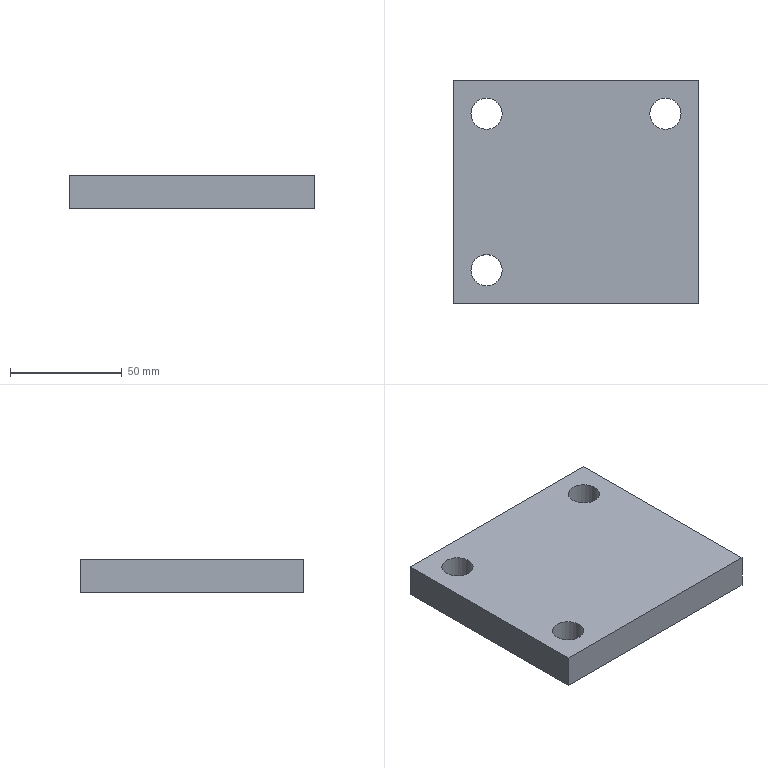Part | NX | features solid 2 | 1 solid | 9 faces | box 110 x 100 x 15 mm | volume 158073 mm3 | plane 6 | cylinder 3 | commonest cylinder face diameters 14 x3
STEP:
#1=CARTESIAN_POINT('',(625.,-751.,-305.));
#2=VERTEX_POINT('',#1);
#3=CARTESIAN_POINT('',(625.,-851.,-305.));
#4=VERTEX_POINT('',#3);
#5=CARTESIAN_POINT('',(625.,-751.,-305.));
#6=DIRECTION('',(0.,1.,0.));
#7=VECTOR('',#6,1000.);
#8=LINE('',#5,#7);
#9=EDGE_CURVE('',#2,#4,#8,.F.);
#10=ORIENTED_EDGE('',*,*,#9,.F.);
#11=CARTESIAN_POINT('',(735.,-751.,-305.));
#12=VERTEX_POINT('',#11);
#13=CARTESIAN_POINT('',(685.,-751.,-305.));
#14=DIRECTION('',(1.,0.,0.));
#15=VECTOR('',#14,1000.);
#16=LINE('',#13,#15);
#17=EDGE_CURVE('',#2,#12,#16,.T.);
#18=ORIENTED_EDGE('',*,*,#17,.T.);
#19=CARTESIAN_POINT('',(735.,-851.,-305.));
#20=VERTEX_POINT('',#19);
#21=CARTESIAN_POINT('',(735.,-842.5,-305.));
#22=DIRECTION('',(0.,-1.,0.));
#23=VECTOR('',#22,1000.);
#24=LINE('',#21,#23);
#25=EDGE_CURVE('',#12,#20,#24,.T.);
#26=ORIENTED_EDGE('',*,*,#25,.T.);
#27=CARTESIAN_POINT('',(685.,-851.,-305.));
#28=DIRECTION('',(1.,0.,0.));
#29=VECTOR('',#28,1000.);
#30=LINE('',#27,#29);
#31=EDGE_CURVE('',#4,#20,#30,.T.);
#32=ORIENTED_EDGE('',*,*,#31,.F.);
#33=EDGE_LOOP('',(#10,#18,#26,#32));
#34=FACE_BOUND('',#33,.T.);
#35=CARTESIAN_POINT('',(633.,-766.,-305.));
#36=VERTEX_POINT('',#35);
#37=CARTESIAN_POINT('',(640.,-766.,-305.));
#38=DIRECTION('',(0.,0.,-1.));
#39=DIRECTION('',(-1.,0.,0.));
#40=AXIS2_PLACEMENT_3D('',#37,#38,#39);
#41=CIRCLE('',#40,7.);
#42=EDGE_CURVE('',#36,#36,#41,.T.);
#43=ORIENTED_EDGE('',*,*,#42,.F.);
#44=EDGE_LOOP('',(#43));
#45=FACE_BOUND('',#44,.T.);
#46=CARTESIAN_POINT('',(713.,-766.,-305.));
#47=VERTEX_POINT('',#46);
#48=CARTESIAN_POINT('',(720.,-766.,-305.));
#49=DIRECTION('',(0.,0.,-1.));
#50=DIRECTION('',(-1.,0.,0.));
#51=AXIS2_PLACEMENT_3D('',#48,#49,#50);
#52=CIRCLE('',#51,7.);
#53=EDGE_CURVE('',#47,#47,#52,.T.);
#54=ORIENTED_EDGE('',*,*,#53,.F.);
#55=EDGE_LOOP('',(#54));
#56=FACE_BOUND('',#55,.T.);
#57=CARTESIAN_POINT('',(633.,-836.,-305.));
#58=VERTEX_POINT('',#57);
#59=CARTESIAN_POINT('',(640.,-836.,-305.));
#60=DIRECTION('',(0.,0.,-1.));
#61=DIRECTION('',(-1.,0.,0.));
#62=AXIS2_PLACEMENT_3D('',#59,#60,#61);
#63=CIRCLE('',#62,7.);
#64=EDGE_CURVE('',#58,#58,#63,.T.);
#65=ORIENTED_EDGE('',*,*,#64,.F.);
#66=EDGE_LOOP('',(#65));
#67=FACE_BOUND('',#66,.T.);
#68=CARTESIAN_POINT('',(685.,-842.5,-305.));
#69=DIRECTION('',(0.,0.,-1.));
#70=DIRECTION('',(1.,0.,0.));
#71=AXIS2_PLACEMENT_3D('',#68,#69,#70);
#72=PLANE('',#71);
#73=ADVANCED_FACE('',(#34,#45,#56,#67),#72,.T.);
#74=CARTESIAN_POINT('',(735.,-751.,-290.));
#75=VERTEX_POINT('',#74);
#76=CARTESIAN_POINT('',(735.,-751.,-305.));
#77=DIRECTION('',(0.,0.,1.));
#78=VECTOR('',#77,1000.);
#79=LINE('',#76,#78);
#80=EDGE_CURVE('',#12,#75,#79,.T.);
#81=ORIENTED_EDGE('',*,*,#80,.T.);
#82=CARTESIAN_POINT('',(735.,-851.,-290.));
#83=VERTEX_POINT('',#82);
#84=CARTESIAN_POINT('',(735.,-842.5,-290.));
#85=DIRECTION('',(0.,-1.,0.));
#86=VECTOR('',#85,1000.);
#87=LINE('',#84,#86);
#88=EDGE_CURVE('',#75,#83,#87,.T.);
#89=ORIENTED_EDGE('',*,*,#88,.T.);
#90=CARTESIAN_POINT('',(735.,-851.,-305.));
#91=DIRECTION('',(0.,0.,1.));
#92=VECTOR('',#91,1000.);
#93=LINE('',#90,#92);
#94=EDGE_CURVE('',#20,#83,#93,.T.);
#95=ORIENTED_EDGE('',*,*,#94,.F.);
#96=ORIENTED_EDGE('',*,*,#25,.F.);
#97=EDGE_LOOP('',(#81,#89,#95,#96));
#98=FACE_BOUND('',#97,.T.);
#99=CARTESIAN_POINT('',(735.,-835.,-31.379));
#100=DIRECTION('',(1.,0.,0.));
#101=DIRECTION('',(0.,0.,-1.));
#102=AXIS2_PLACEMENT_3D('',#99,#100,#101);
#103=PLANE('',#102);
#104=ADVANCED_FACE('',(#98),#103,.T.);
#105=ORIENTED_EDGE('',*,*,#88,.F.);
#106=CARTESIAN_POINT('',(625.,-751.,-290.));
#107=VERTEX_POINT('',#106);
#108=CARTESIAN_POINT('',(685.,-751.,-290.));
#109=DIRECTION('',(1.,0.,0.));
#110=VECTOR('',#109,1000.);
#111=LINE('',#108,#110);
#112=EDGE_CURVE('',#107,#75,#111,.T.);
#113=ORIENTED_EDGE('',*,*,#112,.F.);
#114=CARTESIAN_POINT('',(625.,-851.,-290.));
#115=VERTEX_POINT('',#114);
#116=CARTESIAN_POINT('',(625.,-842.5,-290.));
#117=DIRECTION('',(0.,-1.,0.));
#118=VECTOR('',#117,1000.);
#119=LINE('',#116,#118);
#120=EDGE_CURVE('',#107,#115,#119,.T.);
#121=ORIENTED_EDGE('',*,*,#120,.T.);
#122=CARTESIAN_POINT('',(685.,-851.,-290.));
#123=DIRECTION('',(1.,0.,0.));
#124=VECTOR('',#123,1000.);
#125=LINE('',#122,#124);
#126=EDGE_CURVE('',#115,#83,#125,.T.);
#127=ORIENTED_EDGE('',*,*,#126,.T.);
#128=EDGE_LOOP('',(#105,#113,#121,#127));
#129=FACE_BOUND('',#128,.T.);
#130=CARTESIAN_POINT('',(633.,-836.,-290.));
#131=VERTEX_POINT('',#130);
#132=CARTESIAN_POINT('',(640.,-836.,-290.));
#133=DIRECTION('',(0.,0.,-1.));
#134=DIRECTION('',(-1.,0.,0.));
#135=AXIS2_PLACEMENT_3D('',#132,#133,#134);
#136=CIRCLE('',#135,7.);
#137=EDGE_CURVE('',#131,#131,#136,.T.);
#138=ORIENTED_EDGE('',*,*,#137,.T.);
#139=EDGE_LOOP('',(#138));
#140=FACE_BOUND('',#139,.T.);
#141=CARTESIAN_POINT('',(713.,-766.,-290.));
#142=VERTEX_POINT('',#141);
#143=CARTESIAN_POINT('',(720.,-766.,-290.));
#144=DIRECTION('',(0.,0.,-1.));
#145=DIRECTION('',(-1.,0.,0.));
#146=AXIS2_PLACEMENT_3D('',#143,#144,#145);
#147=CIRCLE('',#146,7.);
#148=EDGE_CURVE('',#142,#142,#147,.T.);
#149=ORIENTED_EDGE('',*,*,#148,.T.);
#150=EDGE_LOOP('',(#149));
#151=FACE_BOUND('',#150,.T.);
#152=CARTESIAN_POINT('',(633.,-766.,-290.));
#153=VERTEX_POINT('',#152);
#154=CARTESIAN_POINT('',(640.,-766.,-290.));
#155=DIRECTION('',(0.,0.,-1.));
#156=DIRECTION('',(-1.,0.,0.));
#157=AXIS2_PLACEMENT_3D('',#154,#155,#156);
#158=CIRCLE('',#157,7.);
#159=EDGE_CURVE('',#153,#153,#158,.T.);
#160=ORIENTED_EDGE('',*,*,#159,.T.);
#161=EDGE_LOOP('',(#160));
#162=FACE_BOUND('',#161,.T.);
#163=CARTESIAN_POINT('',(685.,-842.5,-290.));
#164=DIRECTION('',(0.,0.,-1.));
#165=DIRECTION('',(1.,0.,0.));
#166=AXIS2_PLACEMENT_3D('',#163,#164,#165);
#167=PLANE('',#166);
#168=ADVANCED_FACE('',(#129,#140,#151,#162),#167,.F.);
#169=CARTESIAN_POINT('',(625.,-751.,-355.));
#170=DIRECTION('',(0.,0.,-1.));
#171=VECTOR('',#170,1000.);
#172=LINE('',#169,#171);
#173=EDGE_CURVE('',#2,#107,#172,.F.);
#174=ORIENTED_EDGE('',*,*,#173,.F.);
#175=ORIENTED_EDGE('',*,*,#9,.T.);
#176=CARTESIAN_POINT('',(625.,-851.,-355.));
#177=DIRECTION('',(0.,0.,-1.));
#178=VECTOR('',#177,1000.);
#179=LINE('',#176,#178);
#180=EDGE_CURVE('',#4,#115,#179,.F.);
#181=ORIENTED_EDGE('',*,*,#180,.T.);
#182=ORIENTED_EDGE('',*,*,#120,.F.);
#183=EDGE_LOOP('',(#174,#175,#181,#182));
#184=FACE_BOUND('',#183,.T.);
#185=CARTESIAN_POINT('',(625.,-751.,-355.));
#186=DIRECTION('',(1.,0.,0.));
#187=DIRECTION('',(0.,-1.,0.));
#188=AXIS2_PLACEMENT_3D('',#185,#186,#187);
#189=PLANE('',#188);
#190=ADVANCED_FACE('',(#184),#189,.F.);
#191=ORIENTED_EDGE('',*,*,#126,.F.);
#192=ORIENTED_EDGE('',*,*,#180,.F.);
#193=ORIENTED_EDGE('',*,*,#31,.T.);
#194=ORIENTED_EDGE('',*,*,#94,.T.);
#195=EDGE_LOOP('',(#191,#192,#193,#194));
#196=FACE_BOUND('',#195,.T.);
#197=CARTESIAN_POINT('',(685.,-851.,-305.));
#198=DIRECTION('',(0.,-1.,0.));
#199=DIRECTION('',(1.,0.,0.));
#200=AXIS2_PLACEMENT_3D('',#197,#198,#199);
#201=PLANE('',#200);
#202=ADVANCED_FACE('',(#196),#201,.T.);
#203=ORIENTED_EDGE('',*,*,#112,.T.);
#204=ORIENTED_EDGE('',*,*,#80,.F.);
#205=ORIENTED_EDGE('',*,*,#17,.F.);
#206=ORIENTED_EDGE('',*,*,#173,.T.);
#207=EDGE_LOOP('',(#203,#204,#205,#206));
#208=FACE_BOUND('',#207,.T.);
#209=CARTESIAN_POINT('',(685.,-751.,-305.));
#210=DIRECTION('',(0.,-1.,0.));
#211=DIRECTION('',(1.,0.,0.));
#212=AXIS2_PLACEMENT_3D('',#209,#210,#211);
#213=PLANE('',#212);
#214=ADVANCED_FACE('',(#208),#213,.F.);
#215=ORIENTED_EDGE('',*,*,#42,.T.);
#216=EDGE_LOOP('',(#215));
#217=FACE_BOUND('',#216,.T.);
#218=ORIENTED_EDGE('',*,*,#159,.F.);
#219=EDGE_LOOP('',(#218));
#220=FACE_BOUND('',#219,.T.);
#221=CARTESIAN_POINT('',(640.,-766.,-290.));
#222=DIRECTION('',(0.,0.,-1.));
#223=DIRECTION('',(-1.,0.,0.));
#224=AXIS2_PLACEMENT_3D('',#221,#222,#223);
#225=CYLINDRICAL_SURFACE('',#224,7.);
#226=ADVANCED_FACE('',(#217,#220),#225,.F.);
#227=ORIENTED_EDGE('',*,*,#53,.T.);
#228=EDGE_LOOP('',(#227));
#229=FACE_BOUND('',#228,.T.);
#230=ORIENTED_EDGE('',*,*,#148,.F.);
#231=EDGE_LOOP('',(#230));
#232=FACE_BOUND('',#231,.T.);
#233=CARTESIAN_POINT('',(720.,-766.,-290.));
#234=DIRECTION('',(0.,0.,-1.));
#235=DIRECTION('',(-1.,0.,0.));
#236=AXIS2_PLACEMENT_3D('',#233,#234,#235);
#237=CYLINDRICAL_SURFACE('',#236,7.);
#238=ADVANCED_FACE('',(#229,#232),#237,.F.);
#239=ORIENTED_EDGE('',*,*,#64,.T.);
#240=EDGE_LOOP('',(#239));
#241=FACE_BOUND('',#240,.T.);
#242=ORIENTED_EDGE('',*,*,#137,.F.);
#243=EDGE_LOOP('',(#242));
#244=FACE_BOUND('',#243,.T.);
#245=CARTESIAN_POINT('',(640.,-836.,-290.));
#246=DIRECTION('',(0.,0.,-1.));
#247=DIRECTION('',(-1.,0.,0.));
#248=AXIS2_PLACEMENT_3D('',#245,#246,#247);
#249=CYLINDRICAL_SURFACE('',#248,7.);
#250=ADVANCED_FACE('',(#241,#244),#249,.F.);
#251=CLOSED_SHELL('',(#73,#104,#168,#190,#202,#214,#226,#238,#250));
#252=MANIFOLD_SOLID_BREP('',#251);
#253=(LENGTH_UNIT()NAMED_UNIT(*)SI_UNIT(.MILLI.,.METRE.));
#254=UNCERTAINTY_MEASURE_WITH_UNIT(LENGTH_MEASURE(0.00001),#253,'','');
#255=(NAMED_UNIT(*)PLANE_ANGLE_UNIT()SI_UNIT($,.RADIAN.));
#256=(NAMED_UNIT(*)SI_UNIT($,.STERADIAN.)SOLID_ANGLE_UNIT());
#257=(GEOMETRIC_REPRESENTATION_CONTEXT(3)GLOBAL_UNCERTAINTY_ASSIGNED_CONTEXT((#254))GLOBAL_UNIT_ASSIGNED_CONTEXT((#253,#255,#256))REPRESENTATION_CONTEXT('',''));
#258=ADVANCED_BREP_SHAPE_REPRESENTATION('',(#252),#257);